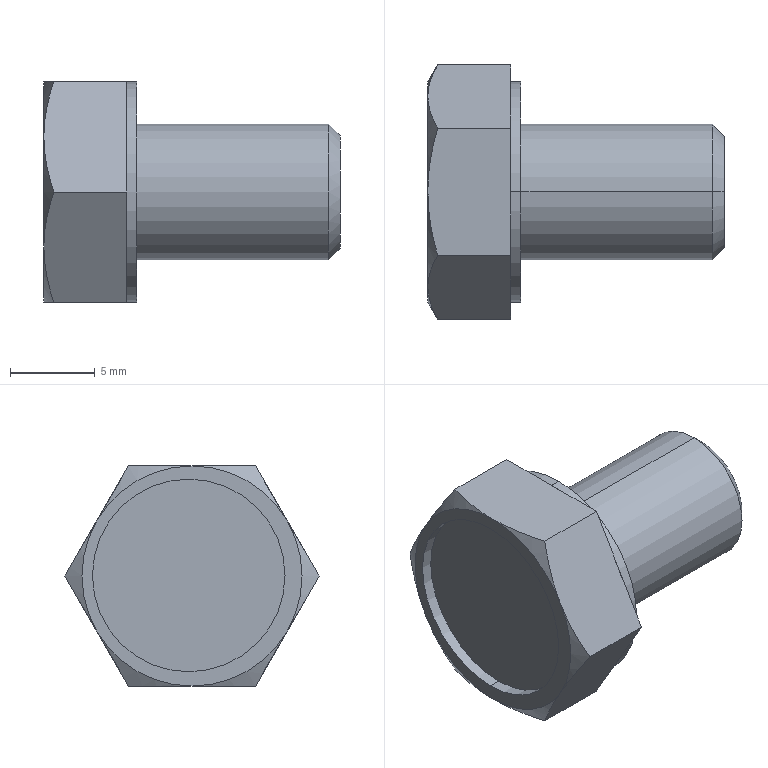Part | STEP file | formed hex screw_am_B18.2.3.2M - Formed hex screw, M8 x 1.25 x 12 --12WN | 1 solid | 30 faces | box 17.5 x 15.011 x 13 mm | volume 1322 mm3 | plane 16 | cone 8 | cylinder 6 | commonest cylinder face diameters 8 x2 11.375 x2 13 x2